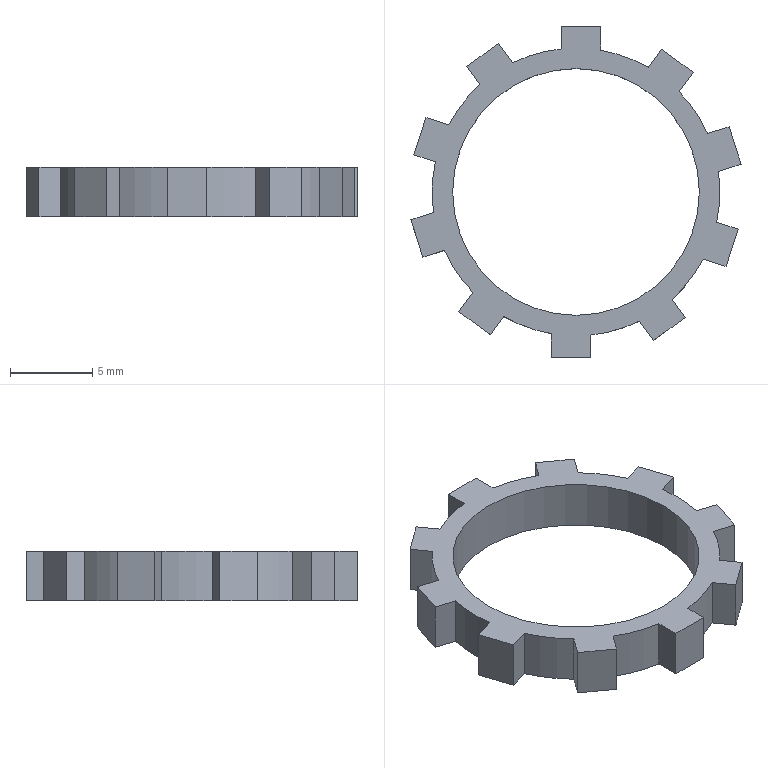Part | NX | features DATUM_CSYS 2, EXTRUDE 1, SKETCH 1 | 1 solid | 43 faces | box 20.095 x 20.159 x 3 mm | volume 289.163 mm3 | plane 32 | cylinder 11 | commonest cylinder face diameters 17.5 x10 15 x1
STEP:
#1=CARTESIAN_POINT('',(-10.047,-1.695,0.));
#2=VERTEX_POINT('',#1);
#3=CARTESIAN_POINT('',(-9.308,-3.971,0.));
#4=VERTEX_POINT('',#3);
#5=CARTESIAN_POINT('',(-10.047,-1.695,0.));
#6=DIRECTION('',(0.309,-0.9511,0.));
#7=VECTOR('',#6,1000.);
#8=LINE('',#5,#7);
#9=EDGE_CURVE('',#2,#4,#8,.T.);
#10=ORIENTED_EDGE('',*,*,#9,.T.);
#11=CARTESIAN_POINT('',(-9.308,-3.971,3.));
#12=VERTEX_POINT('',#11);
#13=CARTESIAN_POINT('',(-9.308,-3.971,3.));
#14=DIRECTION('',(0.,0.,-1.));
#15=VECTOR('',#14,1000.);
#16=LINE('',#13,#15);
#17=EDGE_CURVE('',#12,#4,#16,.T.);
#18=ORIENTED_EDGE('',*,*,#17,.F.);
#19=CARTESIAN_POINT('',(-10.047,-1.695,3.));
#20=VERTEX_POINT('',#19);
#21=CARTESIAN_POINT('',(-10.047,-1.695,3.));
#22=DIRECTION('',(0.309,-0.9511,0.));
#23=VECTOR('',#22,1000.);
#24=LINE('',#21,#23);
#25=EDGE_CURVE('',#20,#12,#24,.T.);
#26=ORIENTED_EDGE('',*,*,#25,.F.);
#27=CARTESIAN_POINT('',(-10.047,-1.695,3.));
#28=DIRECTION('',(0.,0.,-1.));
#29=VECTOR('',#28,1000.);
#30=LINE('',#27,#29);
#31=EDGE_CURVE('',#20,#2,#30,.T.);
#32=ORIENTED_EDGE('',*,*,#31,.T.);
#33=EDGE_LOOP('',(#10,#18,#26,#32));
#34=FACE_BOUND('',#33,.T.);
#35=CARTESIAN_POINT('',(-10.047,-1.695,3.));
#36=DIRECTION('',(0.9511,0.309,0.));
#37=DIRECTION('',(-0.309,0.9511,0.));
#38=AXIS2_PLACEMENT_3D('',#35,#36,#37);
#39=PLANE('',#38);
#40=ADVANCED_FACE('',(#34),#39,.F.);
#41=CARTESIAN_POINT('',(-7.999,-3.545,0.));
#42=VERTEX_POINT('',#41);
#43=CARTESIAN_POINT('',(-9.308,-3.971,0.));
#44=DIRECTION('',(0.9511,0.309,0.));
#45=VECTOR('',#44,1000.);
#46=LINE('',#43,#45);
#47=EDGE_CURVE('',#4,#42,#46,.T.);
#48=ORIENTED_EDGE('',*,*,#47,.T.);
#49=CARTESIAN_POINT('',(-7.999,-3.545,3.));
#50=VERTEX_POINT('',#49);
#51=CARTESIAN_POINT('',(-7.999,-3.545,3.));
#52=DIRECTION('',(0.,0.,-1.));
#53=VECTOR('',#52,1000.);
#54=LINE('',#51,#53);
#55=EDGE_CURVE('',#50,#42,#54,.T.);
#56=ORIENTED_EDGE('',*,*,#55,.F.);
#57=CARTESIAN_POINT('',(-9.308,-3.971,3.));
#58=DIRECTION('',(0.9511,0.309,0.));
#59=VECTOR('',#58,1000.);
#60=LINE('',#57,#59);
#61=EDGE_CURVE('',#12,#50,#60,.T.);
#62=ORIENTED_EDGE('',*,*,#61,.F.);
#63=ORIENTED_EDGE('',*,*,#17,.T.);
#64=EDGE_LOOP('',(#48,#56,#62,#63));
#65=FACE_BOUND('',#64,.T.);
#66=CARTESIAN_POINT('',(-9.308,-3.971,3.));
#67=DIRECTION('',(-0.309,0.9511,0.));
#68=DIRECTION('',(-0.9511,-0.309,0.));
#69=AXIS2_PLACEMENT_3D('',#66,#67,#68);
#70=PLANE('',#69);
#71=ADVANCED_FACE('',(#65),#70,.F.);
#72=CARTESIAN_POINT('',(-6.275,-6.098,0.));
#73=VERTEX_POINT('',#72);
#74=CARTESIAN_POINT('',(0.,0.,0.));
#75=DIRECTION('',(0.,0.,1.));
#76=DIRECTION('',(1.,0.,0.));
#77=AXIS2_PLACEMENT_3D('',#74,#75,#76);
#78=CIRCLE('',#77,8.75);
#79=EDGE_CURVE('',#42,#73,#78,.T.);
#80=ORIENTED_EDGE('',*,*,#79,.T.);
#81=CARTESIAN_POINT('',(-6.275,-6.098,3.));
#82=VERTEX_POINT('',#81);
#83=CARTESIAN_POINT('',(-6.275,-6.098,3.));
#84=DIRECTION('',(0.,0.,-1.));
#85=VECTOR('',#84,1000.);
#86=LINE('',#83,#85);
#87=EDGE_CURVE('',#82,#73,#86,.T.);
#88=ORIENTED_EDGE('',*,*,#87,.F.);
#89=CARTESIAN_POINT('',(0.,0.,3.));
#90=DIRECTION('',(0.,0.,1.));
#91=DIRECTION('',(1.,0.,0.));
#92=AXIS2_PLACEMENT_3D('',#89,#90,#91);
#93=CIRCLE('',#92,8.75);
#94=EDGE_CURVE('',#50,#82,#93,.T.);
#95=ORIENTED_EDGE('',*,*,#94,.F.);
#96=ORIENTED_EDGE('',*,*,#55,.T.);
#97=EDGE_LOOP('',(#80,#88,#95,#96));
#98=FACE_BOUND('',#97,.T.);
#99=CARTESIAN_POINT('',(0.,0.,3.));
#100=DIRECTION('',(0.,0.,-1.));
#101=DIRECTION('',(-1.,0.,0.));
#102=AXIS2_PLACEMENT_3D('',#99,#100,#101);
#103=CYLINDRICAL_SURFACE('',#102,8.75);
#104=ADVANCED_FACE('',(#98),#103,.T.);
#105=CARTESIAN_POINT('',(-7.132,-7.277,0.));
#106=VERTEX_POINT('',#105);
#107=CARTESIAN_POINT('',(-6.275,-6.098,0.));
#108=DIRECTION('',(-0.5878,-0.809,0.));
#109=VECTOR('',#108,1000.);
#110=LINE('',#107,#109);
#111=EDGE_CURVE('',#73,#106,#110,.T.);
#112=ORIENTED_EDGE('',*,*,#111,.T.);
#113=CARTESIAN_POINT('',(-7.132,-7.277,3.));
#114=VERTEX_POINT('',#113);
#115=CARTESIAN_POINT('',(-7.132,-7.277,3.));
#116=DIRECTION('',(0.,0.,-1.));
#117=VECTOR('',#116,1000.);
#118=LINE('',#115,#117);
#119=EDGE_CURVE('',#114,#106,#118,.T.);
#120=ORIENTED_EDGE('',*,*,#119,.F.);
#121=CARTESIAN_POINT('',(-6.275,-6.098,3.));
#122=DIRECTION('',(-0.5878,-0.809,0.));
#123=VECTOR('',#122,1000.);
#124=LINE('',#121,#123);
#125=EDGE_CURVE('',#82,#114,#124,.T.);
#126=ORIENTED_EDGE('',*,*,#125,.F.);
#127=ORIENTED_EDGE('',*,*,#87,.T.);
#128=EDGE_LOOP('',(#112,#120,#126,#127));
#129=FACE_BOUND('',#128,.T.);
#130=CARTESIAN_POINT('',(-6.275,-6.098,3.));
#131=DIRECTION('',(0.809,-0.5878,0.));
#132=DIRECTION('',(0.5878,0.809,0.));
#133=AXIS2_PLACEMENT_3D('',#130,#131,#132);
#134=PLANE('',#133);
#135=ADVANCED_FACE('',(#129),#134,.F.);
#136=CARTESIAN_POINT('',(-5.196,-8.683,0.));
#137=VERTEX_POINT('',#136);
#138=CARTESIAN_POINT('',(-7.132,-7.277,0.));
#139=DIRECTION('',(0.809,-0.5878,0.));
#140=VECTOR('',#139,1000.);
#141=LINE('',#138,#140);
#142=EDGE_CURVE('',#106,#137,#141,.T.);
#143=ORIENTED_EDGE('',*,*,#142,.T.);
#144=CARTESIAN_POINT('',(-5.196,-8.683,3.));
#145=VERTEX_POINT('',#144);
#146=CARTESIAN_POINT('',(-5.196,-8.683,3.));
#147=DIRECTION('',(0.,0.,-1.));
#148=VECTOR('',#147,1000.);
#149=LINE('',#146,#148);
#150=EDGE_CURVE('',#145,#137,#149,.T.);
#151=ORIENTED_EDGE('',*,*,#150,.F.);
#152=CARTESIAN_POINT('',(-7.132,-7.277,3.));
#153=DIRECTION('',(0.809,-0.5878,0.));
#154=VECTOR('',#153,1000.);
#155=LINE('',#152,#154);
#156=EDGE_CURVE('',#114,#145,#155,.T.);
#157=ORIENTED_EDGE('',*,*,#156,.F.);
#158=ORIENTED_EDGE('',*,*,#119,.T.);
#159=EDGE_LOOP('',(#143,#151,#157,#158));
#160=FACE_BOUND('',#159,.T.);
#161=CARTESIAN_POINT('',(-7.132,-7.277,3.));
#162=DIRECTION('',(0.5878,0.809,0.));
#163=DIRECTION('',(-0.809,0.5878,0.));
#164=AXIS2_PLACEMENT_3D('',#161,#162,#163);
#165=PLANE('',#164);
#166=ADVANCED_FACE('',(#160),#165,.F.);
#167=CARTESIAN_POINT('',(-4.388,-7.57,0.));
#168=VERTEX_POINT('',#167);
#169=CARTESIAN_POINT('',(-5.196,-8.683,0.));
#170=DIRECTION('',(0.5878,0.809,0.));
#171=VECTOR('',#170,1000.);
#172=LINE('',#169,#171);
#173=EDGE_CURVE('',#137,#168,#172,.T.);
#174=ORIENTED_EDGE('',*,*,#173,.T.);
#175=CARTESIAN_POINT('',(-4.388,-7.57,3.));
#176=VERTEX_POINT('',#175);
#177=CARTESIAN_POINT('',(-4.388,-7.57,3.));
#178=DIRECTION('',(0.,0.,-1.));
#179=VECTOR('',#178,1000.);
#180=LINE('',#177,#179);
#181=EDGE_CURVE('',#176,#168,#180,.T.);
#182=ORIENTED_EDGE('',*,*,#181,.F.);
#183=CARTESIAN_POINT('',(-5.196,-8.683,3.));
#184=DIRECTION('',(0.5878,0.809,0.));
#185=VECTOR('',#184,1000.);
#186=LINE('',#183,#185);
#187=EDGE_CURVE('',#145,#176,#186,.T.);
#188=ORIENTED_EDGE('',*,*,#187,.F.);
#189=ORIENTED_EDGE('',*,*,#150,.T.);
#190=EDGE_LOOP('',(#174,#182,#188,#189));
#191=FACE_BOUND('',#190,.T.);
#192=CARTESIAN_POINT('',(-5.196,-8.683,3.));
#193=DIRECTION('',(-0.809,0.5878,0.));
#194=DIRECTION('',(-0.5878,-0.809,0.));
#195=AXIS2_PLACEMENT_3D('',#192,#193,#194);
#196=PLANE('',#195);
#197=ADVANCED_FACE('',(#191),#196,.F.);
#198=CARTESIAN_POINT('',(-1.492,-8.622,0.));
#199=VERTEX_POINT('',#198);
#200=CARTESIAN_POINT('',(0.,0.,0.));
#201=DIRECTION('',(0.,0.,1.));
#202=DIRECTION('',(1.,0.,0.));
#203=AXIS2_PLACEMENT_3D('',#200,#201,#202);
#204=CIRCLE('',#203,8.75);
#205=EDGE_CURVE('',#168,#199,#204,.T.);
#206=ORIENTED_EDGE('',*,*,#205,.T.);
#207=CARTESIAN_POINT('',(-1.492,-8.622,3.));
#208=VERTEX_POINT('',#207);
#209=CARTESIAN_POINT('',(-1.492,-8.622,3.));
#210=DIRECTION('',(0.,0.,-1.));
#211=VECTOR('',#210,1000.);
#212=LINE('',#209,#211);
#213=EDGE_CURVE('',#208,#199,#212,.T.);
#214=ORIENTED_EDGE('',*,*,#213,.F.);
#215=CARTESIAN_POINT('',(0.,0.,3.));
#216=DIRECTION('',(0.,0.,1.));
#217=DIRECTION('',(1.,0.,0.));
#218=AXIS2_PLACEMENT_3D('',#215,#216,#217);
#219=CIRCLE('',#218,8.75);
#220=EDGE_CURVE('',#176,#208,#219,.T.);
#221=ORIENTED_EDGE('',*,*,#220,.F.);
#222=ORIENTED_EDGE('',*,*,#181,.T.);
#223=EDGE_LOOP('',(#206,#214,#221,#222));
#224=FACE_BOUND('',#223,.T.);
#225=CARTESIAN_POINT('',(0.,0.,3.));
#226=DIRECTION('',(0.,0.,-1.));
#227=DIRECTION('',(-1.,0.,0.));
#228=AXIS2_PLACEMENT_3D('',#225,#226,#227);
#229=CYLINDRICAL_SURFACE('',#228,8.75);
#230=ADVANCED_FACE('',(#224),#229,.T.);
#231=CARTESIAN_POINT('',(-1.492,-10.079,0.));
#232=VERTEX_POINT('',#231);
#233=CARTESIAN_POINT('',(-1.492,-8.622,0.));
#234=DIRECTION('',(0.,-1.,0.));
#235=VECTOR('',#234,1000.);
#236=LINE('',#233,#235);
#237=EDGE_CURVE('',#199,#232,#236,.T.);
#238=ORIENTED_EDGE('',*,*,#237,.T.);
#239=CARTESIAN_POINT('',(-1.492,-10.079,3.));
#240=VERTEX_POINT('',#239);
#241=CARTESIAN_POINT('',(-1.492,-10.079,3.));
#242=DIRECTION('',(0.,0.,-1.));
#243=VECTOR('',#242,1000.);
#244=LINE('',#241,#243);
#245=EDGE_CURVE('',#240,#232,#244,.T.);
#246=ORIENTED_EDGE('',*,*,#245,.F.);
#247=CARTESIAN_POINT('',(-1.492,-8.622,3.));
#248=DIRECTION('',(0.,-1.,0.));
#249=VECTOR('',#248,1000.);
#250=LINE('',#247,#249);
#251=EDGE_CURVE('',#208,#240,#250,.T.);
#252=ORIENTED_EDGE('',*,*,#251,.F.);
#253=ORIENTED_EDGE('',*,*,#213,.T.);
#254=EDGE_LOOP('',(#238,#246,#252,#253));
#255=FACE_BOUND('',#254,.T.);
#256=CARTESIAN_POINT('',(-1.492,-8.622,3.));
#257=DIRECTION('',(1.,0.,0.));
#258=DIRECTION('',(0.,1.,0.));
#259=AXIS2_PLACEMENT_3D('',#256,#257,#258);
#260=PLANE('',#259);
#261=ADVANCED_FACE('',(#255),#260,.F.);
#262=CARTESIAN_POINT('',(0.9,-10.079,0.));
#263=VERTEX_POINT('',#262);
#264=CARTESIAN_POINT('',(-1.492,-10.079,0.));
#265=DIRECTION('',(1.,0.,0.));
#266=VECTOR('',#265,1000.);
#267=LINE('',#264,#266);
#268=EDGE_CURVE('',#232,#263,#267,.T.);
#269=ORIENTED_EDGE('',*,*,#268,.T.);
#270=CARTESIAN_POINT('',(0.9,-10.079,3.));
#271=VERTEX_POINT('',#270);
#272=CARTESIAN_POINT('',(0.9,-10.079,3.));
#273=DIRECTION('',(0.,0.,-1.));
#274=VECTOR('',#273,1000.);
#275=LINE('',#272,#274);
#276=EDGE_CURVE('',#271,#263,#275,.T.);
#277=ORIENTED_EDGE('',*,*,#276,.F.);
#278=CARTESIAN_POINT('',(-1.492,-10.079,3.));
#279=DIRECTION('',(1.,0.,0.));
#280=VECTOR('',#279,1000.);
#281=LINE('',#278,#280);
#282=EDGE_CURVE('',#240,#271,#281,.T.);
#283=ORIENTED_EDGE('',*,*,#282,.F.);
#284=ORIENTED_EDGE('',*,*,#245,.T.);
#285=EDGE_LOOP('',(#269,#277,#283,#284));
#286=FACE_BOUND('',#285,.T.);
#287=CARTESIAN_POINT('',(-1.492,-10.079,3.));
#288=DIRECTION('',(0.,1.,0.));
#289=DIRECTION('',(0.,0.,1.));
#290=AXIS2_PLACEMENT_3D('',#287,#288,#289);
#291=PLANE('',#290);
#292=ADVANCED_FACE('',(#286),#291,.F.);
#293=CARTESIAN_POINT('',(0.9,-8.703,0.));
#294=VERTEX_POINT('',#293);
#295=CARTESIAN_POINT('',(0.9,-10.079,0.));
#296=DIRECTION('',(0.,1.,0.));
#297=VECTOR('',#296,1000.);
#298=LINE('',#295,#297);
#299=EDGE_CURVE('',#263,#294,#298,.T.);
#300=ORIENTED_EDGE('',*,*,#299,.T.);
#301=CARTESIAN_POINT('',(0.9,-8.703,3.));
#302=VERTEX_POINT('',#301);
#303=CARTESIAN_POINT('',(0.9,-8.703,3.));
#304=DIRECTION('',(0.,0.,-1.));
#305=VECTOR('',#304,1000.);
#306=LINE('',#303,#305);
#307=EDGE_CURVE('',#302,#294,#306,.T.);
#308=ORIENTED_EDGE('',*,*,#307,.F.);
#309=CARTESIAN_POINT('',(0.9,-10.079,3.));
#310=DIRECTION('',(0.,1.,0.));
#311=VECTOR('',#310,1000.);
#312=LINE('',#309,#311);
#313=EDGE_CURVE('',#271,#302,#312,.T.);
#314=ORIENTED_EDGE('',*,*,#313,.F.);
#315=ORIENTED_EDGE('',*,*,#276,.T.);
#316=EDGE_LOOP('',(#300,#308,#314,#315));
#317=FACE_BOUND('',#316,.T.);
#318=CARTESIAN_POINT('',(0.9,-10.079,3.));
#319=DIRECTION('',(-1.,0.,0.));
#320=DIRECTION('',(0.,-1.,0.));
#321=AXIS2_PLACEMENT_3D('',#318,#319,#320);
#322=PLANE('',#321);
#323=ADVANCED_FACE('',(#317),#322,.F.);
#324=CARTESIAN_POINT('',(3.86,-7.852,0.));
#325=VERTEX_POINT('',#324);
#326=CARTESIAN_POINT('',(0.,0.,0.));
#327=DIRECTION('',(0.,0.,1.));
#328=DIRECTION('',(1.,0.,0.));
#329=AXIS2_PLACEMENT_3D('',#326,#327,#328);
#330=CIRCLE('',#329,8.75);
#331=EDGE_CURVE('',#294,#325,#330,.T.);
#332=ORIENTED_EDGE('',*,*,#331,.T.);
#333=CARTESIAN_POINT('',(3.86,-7.852,3.));
#334=VERTEX_POINT('',#333);
#335=CARTESIAN_POINT('',(3.86,-7.852,3.));
#336=DIRECTION('',(0.,0.,-1.));
#337=VECTOR('',#336,1000.);
#338=LINE('',#335,#337);
#339=EDGE_CURVE('',#334,#325,#338,.T.);
#340=ORIENTED_EDGE('',*,*,#339,.F.);
#341=CARTESIAN_POINT('',(0.,0.,3.));
#342=DIRECTION('',(0.,0.,1.));
#343=DIRECTION('',(1.,0.,0.));
#344=AXIS2_PLACEMENT_3D('',#341,#342,#343);
#345=CIRCLE('',#344,8.75);
#346=EDGE_CURVE('',#302,#334,#345,.T.);
#347=ORIENTED_EDGE('',*,*,#346,.F.);
#348=ORIENTED_EDGE('',*,*,#307,.T.);
#349=EDGE_LOOP('',(#332,#340,#347,#348));
#350=FACE_BOUND('',#349,.T.);
#351=CARTESIAN_POINT('',(0.,0.,3.));
#352=DIRECTION('',(0.,0.,-1.));
#353=DIRECTION('',(-1.,0.,0.));
#354=AXIS2_PLACEMENT_3D('',#351,#352,#353);
#355=CYLINDRICAL_SURFACE('',#354,8.75);
#356=ADVANCED_FACE('',(#350),#355,.T.);
#357=CARTESIAN_POINT('',(4.717,-9.032,0.));
#358=VERTEX_POINT('',#357);
#359=CARTESIAN_POINT('',(3.86,-7.852,0.));
#360=DIRECTION('',(0.5878,-0.809,0.));
#361=VECTOR('',#360,1000.);
#362=LINE('',#359,#361);
#363=EDGE_CURVE('',#325,#358,#362,.T.);
#364=ORIENTED_EDGE('',*,*,#363,.T.);
#365=CARTESIAN_POINT('',(4.717,-9.032,3.));
#366=VERTEX_POINT('',#365);
#367=CARTESIAN_POINT('',(4.717,-9.032,3.));
#368=DIRECTION('',(0.,0.,-1.));
#369=VECTOR('',#368,1000.);
#370=LINE('',#367,#369);
#371=EDGE_CURVE('',#366,#358,#370,.T.);
#372=ORIENTED_EDGE('',*,*,#371,.F.);
#373=CARTESIAN_POINT('',(3.86,-7.852,3.));
#374=DIRECTION('',(0.5878,-0.809,0.));
#375=VECTOR('',#374,1000.);
#376=LINE('',#373,#375);
#377=EDGE_CURVE('',#334,#366,#376,.T.);
#378=ORIENTED_EDGE('',*,*,#377,.F.);
#379=ORIENTED_EDGE('',*,*,#339,.T.);
#380=EDGE_LOOP('',(#364,#372,#378,#379));
#381=FACE_BOUND('',#380,.T.);
#382=CARTESIAN_POINT('',(3.86,-7.852,3.));
#383=DIRECTION('',(0.809,0.5878,0.));
#384=DIRECTION('',(-0.5878,0.809,0.));
#385=AXIS2_PLACEMENT_3D('',#382,#383,#384);
#386=PLANE('',#385);
#387=ADVANCED_FACE('',(#381),#386,.F.);
#388=CARTESIAN_POINT('',(6.653,-7.625,0.));
#389=VERTEX_POINT('',#388);
#390=CARTESIAN_POINT('',(4.717,-9.032,0.));
#391=DIRECTION('',(0.809,0.5878,0.));
#392=VECTOR('',#391,1000.);
#393=LINE('',#390,#392);
#394=EDGE_CURVE('',#358,#389,#393,.T.);
#395=ORIENTED_EDGE('',*,*,#394,.T.);
#396=CARTESIAN_POINT('',(6.653,-7.625,3.));
#397=VERTEX_POINT('',#396);
#398=CARTESIAN_POINT('',(6.653,-7.625,3.));
#399=DIRECTION('',(0.,0.,-1.));
#400=VECTOR('',#399,1000.);
#401=LINE('',#398,#400);
#402=EDGE_CURVE('',#397,#389,#401,.T.);
#403=ORIENTED_EDGE('',*,*,#402,.F.);
#404=CARTESIAN_POINT('',(4.717,-9.032,3.));
#405=DIRECTION('',(0.809,0.5878,0.));
#406=VECTOR('',#405,1000.);
#407=LINE('',#404,#406);
#408=EDGE_CURVE('',#366,#397,#407,.T.);
#409=ORIENTED_EDGE('',*,*,#408,.F.);
#410=ORIENTED_EDGE('',*,*,#371,.T.);
#411=EDGE_LOOP('',(#395,#403,#409,#410));
#412=FACE_BOUND('',#411,.T.);
#413=CARTESIAN_POINT('',(4.717,-9.032,3.));
#414=DIRECTION('',(-0.5878,0.809,0.));
#415=DIRECTION('',(-0.809,-0.5878,0.));
#416=AXIS2_PLACEMENT_3D('',#413,#414,#415);
#417=PLANE('',#416);
#418=ADVANCED_FACE('',(#412),#417,.F.);
#419=CARTESIAN_POINT('',(5.844,-6.512,0.));
#420=VERTEX_POINT('',#419);
#421=CARTESIAN_POINT('',(6.653,-7.625,0.));
#422=DIRECTION('',(-0.5878,0.809,0.));
#423=VECTOR('',#422,1000.);
#424=LINE('',#421,#423);
#425=EDGE_CURVE('',#389,#420,#424,.T.);
#426=ORIENTED_EDGE('',*,*,#425,.T.);
#427=CARTESIAN_POINT('',(5.844,-6.512,3.));
#428=VERTEX_POINT('',#427);
#429=CARTESIAN_POINT('',(5.844,-6.512,3.));
#430=DIRECTION('',(0.,0.,-1.));
#431=VECTOR('',#430,1000.);
#432=LINE('',#429,#431);
#433=EDGE_CURVE('',#428,#420,#432,.T.);
#434=ORIENTED_EDGE('',*,*,#433,.F.);
#435=CARTESIAN_POINT('',(6.653,-7.625,3.));
#436=DIRECTION('',(-0.5878,0.809,0.));
#437=VECTOR('',#436,1000.);
#438=LINE('',#435,#437);
#439=EDGE_CURVE('',#397,#428,#438,.T.);
#440=ORIENTED_EDGE('',*,*,#439,.F.);
#441=ORIENTED_EDGE('',*,*,#402,.T.);
#442=EDGE_LOOP('',(#426,#434,#440,#441));
#443=FACE_BOUND('',#442,.T.);
#444=CARTESIAN_POINT('',(6.653,-7.625,3.));
#445=DIRECTION('',(-0.809,-0.5878,0.));
#446=DIRECTION('',(0.5878,-0.809,0.));
#447=AXIS2_PLACEMENT_3D('',#444,#445,#446);
#448=PLANE('',#447);
#449=ADVANCED_FACE('',(#443),#448,.F.);
#450=CARTESIAN_POINT('',(7.738,-4.084,0.));
#451=VERTEX_POINT('',#450);
#452=CARTESIAN_POINT('',(0.,0.,0.));
#453=DIRECTION('',(0.,0.,1.));
#454=DIRECTION('',(1.,0.,0.));
#455=AXIS2_PLACEMENT_3D('',#452,#453,#454);
#456=CIRCLE('',#455,8.75);
#457=EDGE_CURVE('',#420,#451,#456,.T.);
#458=ORIENTED_EDGE('',*,*,#457,.T.);
#459=CARTESIAN_POINT('',(7.738,-4.084,3.));
#460=VERTEX_POINT('',#459);
#461=CARTESIAN_POINT('',(7.738,-4.084,3.));
#462=DIRECTION('',(0.,0.,-1.));
#463=VECTOR('',#462,1000.);
#464=LINE('',#461,#463);
#465=EDGE_CURVE('',#460,#451,#464,.T.);
#466=ORIENTED_EDGE('',*,*,#465,.F.);
#467=CARTESIAN_POINT('',(0.,0.,3.));
#468=DIRECTION('',(0.,0.,1.));
#469=DIRECTION('',(1.,0.,0.));
#470=AXIS2_PLACEMENT_3D('',#467,#468,#469);
#471=CIRCLE('',#470,8.75);
#472=EDGE_CURVE('',#428,#460,#471,.T.);
#473=ORIENTED_EDGE('',*,*,#472,.F.);
#474=ORIENTED_EDGE('',*,*,#433,.T.);
#475=EDGE_LOOP('',(#458,#466,#473,#474));
#476=FACE_BOUND('',#475,.T.);
#477=CARTESIAN_POINT('',(0.,0.,3.));
#478=DIRECTION('',(0.,0.,-1.));
#479=DIRECTION('',(-1.,0.,0.));
#480=AXIS2_PLACEMENT_3D('',#477,#478,#479);
#481=CYLINDRICAL_SURFACE('',#480,8.75);
#482=ADVANCED_FACE('',(#476),#481,.T.);
#483=CARTESIAN_POINT('',(9.125,-4.534,0.));
#484=VERTEX_POINT('',#483);
#485=CARTESIAN_POINT('',(7.738,-4.084,0.));
#486=DIRECTION('',(0.9511,-0.309,0.));
#487=VECTOR('',#486,1000.);
#488=LINE('',#485,#487);
#489=EDGE_CURVE('',#451,#484,#488,.T.);
#490=ORIENTED_EDGE('',*,*,#489,.T.);
#491=CARTESIAN_POINT('',(9.125,-4.534,3.));
#492=VERTEX_POINT('',#491);
#493=CARTESIAN_POINT('',(9.125,-4.534,3.));
#494=DIRECTION('',(0.,0.,-1.));
#495=VECTOR('',#494,1000.);
#496=LINE('',#493,#495);
#497=EDGE_CURVE('',#492,#484,#496,.T.);
#498=ORIENTED_EDGE('',*,*,#497,.F.);
#499=CARTESIAN_POINT('',(7.738,-4.084,3.));
#500=DIRECTION('',(0.9511,-0.309,0.));
#501=VECTOR('',#500,1000.);
#502=LINE('',#499,#501);
#503=EDGE_CURVE('',#460,#492,#502,.T.);
#504=ORIENTED_EDGE('',*,*,#503,.F.);
#505=ORIENTED_EDGE('',*,*,#465,.T.);
#506=EDGE_LOOP('',(#490,#498,#504,#505));
#507=FACE_BOUND('',#506,.T.);
#508=CARTESIAN_POINT('',(7.738,-4.084,3.));
#509=DIRECTION('',(0.309,0.9511,0.));
#510=DIRECTION('',(-0.9511,0.309,0.));
#511=AXIS2_PLACEMENT_3D('',#508,#509,#510);
#512=PLANE('',#511);
#513=ADVANCED_FACE('',(#507),#512,.F.);
#514=CARTESIAN_POINT('',(9.864,-2.259,0.));
#515=VERTEX_POINT('',#514);
#516=CARTESIAN_POINT('',(9.125,-4.534,0.));
#517=DIRECTION('',(0.309,0.9511,0.));
#518=VECTOR('',#517,1000.);
#519=LINE('',#516,#518);
#520=EDGE_CURVE('',#484,#515,#519,.T.);
#521=ORIENTED_EDGE('',*,*,#520,.T.);
#522=CARTESIAN_POINT('',(9.864,-2.259,3.));
#523=VERTEX_POINT('',#522);
#524=CARTESIAN_POINT('',(9.864,-2.259,3.));
#525=DIRECTION('',(0.,0.,-1.));
#526=VECTOR('',#525,1000.);
#527=LINE('',#524,#526);
#528=EDGE_CURVE('',#523,#515,#527,.T.);
#529=ORIENTED_EDGE('',*,*,#528,.F.);
#530=CARTESIAN_POINT('',(9.125,-4.534,3.));
#531=DIRECTION('',(0.309,0.9511,0.));
#532=VECTOR('',#531,1000.);
#533=LINE('',#530,#532);
#534=EDGE_CURVE('',#492,#523,#533,.T.);
#535=ORIENTED_EDGE('',*,*,#534,.F.);
#536=ORIENTED_EDGE('',*,*,#497,.T.);
#537=EDGE_LOOP('',(#521,#529,#535,#536));
#538=FACE_BOUND('',#537,.T.);
#539=CARTESIAN_POINT('',(9.125,-4.534,3.));
#540=DIRECTION('',(-0.9511,0.309,0.));
#541=DIRECTION('',(-0.309,-0.9511,0.));
#542=AXIS2_PLACEMENT_3D('',#539,#540,#541);
#543=PLANE('',#542);
#544=ADVANCED_FACE('',(#538),#543,.F.);
#545=CARTESIAN_POINT('',(8.555,-1.834,0.));
#546=VERTEX_POINT('',#545);
#547=CARTESIAN_POINT('',(9.864,-2.259,0.));
#548=DIRECTION('',(-0.9511,0.309,0.));
#549=VECTOR('',#548,1000.);
#550=LINE('',#547,#549);
#551=EDGE_CURVE('',#515,#546,#550,.T.);
#552=ORIENTED_EDGE('',*,*,#551,.T.);
#553=CARTESIAN_POINT('',(8.555,-1.834,3.));
#554=VERTEX_POINT('',#553);
#555=CARTESIAN_POINT('',(8.555,-1.834,3.));
#556=DIRECTION('',(0.,0.,-1.));
#557=VECTOR('',#556,1000.);
#558=LINE('',#555,#557);
#559=EDGE_CURVE('',#554,#546,#558,.T.);
#560=ORIENTED_EDGE('',*,*,#559,.F.);
#561=CARTESIAN_POINT('',(9.864,-2.259,3.));
#562=DIRECTION('',(-0.9511,0.309,0.));
#563=VECTOR('',#562,1000.);
#564=LINE('',#561,#563);
#565=EDGE_CURVE('',#523,#554,#564,.T.);
#566=ORIENTED_EDGE('',*,*,#565,.F.);
#567=ORIENTED_EDGE('',*,*,#528,.T.);
#568=EDGE_LOOP('',(#552,#560,#566,#567));
#569=FACE_BOUND('',#568,.T.);
#570=CARTESIAN_POINT('',(9.864,-2.259,3.));
#571=DIRECTION('',(-0.309,-0.9511,0.));
#572=DIRECTION('',(0.9511,-0.309,0.));
#573=AXIS2_PLACEMENT_3D('',#570,#571,#572);
#574=PLANE('',#573);
#575=ADVANCED_FACE('',(#569),#574,.F.);
#576=CARTESIAN_POINT('',(8.661,1.245,0.));
#577=VERTEX_POINT('',#576);
#578=CARTESIAN_POINT('',(0.,0.,0.));
#579=DIRECTION('',(0.,0.,1.));
#580=DIRECTION('',(1.,0.,0.));
#581=AXIS2_PLACEMENT_3D('',#578,#579,#580);
#582=CIRCLE('',#581,8.75);
#583=EDGE_CURVE('',#546,#577,#582,.T.);
#584=ORIENTED_EDGE('',*,*,#583,.T.);
#585=CARTESIAN_POINT('',(8.661,1.245,3.));
#586=VERTEX_POINT('',#585);
#587=CARTESIAN_POINT('',(8.661,1.245,3.));
#588=DIRECTION('',(0.,0.,-1.));
#589=VECTOR('',#588,1000.);
#590=LINE('',#587,#589);
#591=EDGE_CURVE('',#586,#577,#590,.T.);
#592=ORIENTED_EDGE('',*,*,#591,.F.);
#593=CARTESIAN_POINT('',(0.,0.,3.));
#594=DIRECTION('',(0.,0.,1.));
#595=DIRECTION('',(1.,0.,0.));
#596=AXIS2_PLACEMENT_3D('',#593,#594,#595);
#597=CIRCLE('',#596,8.75);
#598=EDGE_CURVE('',#554,#586,#597,.T.);
#599=ORIENTED_EDGE('',*,*,#598,.F.);
#600=ORIENTED_EDGE('',*,*,#559,.T.);
#601=EDGE_LOOP('',(#584,#592,#599,#600));
#602=FACE_BOUND('',#601,.T.);
#603=CARTESIAN_POINT('',(0.,0.,3.));
#604=DIRECTION('',(0.,0.,-1.));
#605=DIRECTION('',(-1.,0.,0.));
#606=AXIS2_PLACEMENT_3D('',#603,#604,#605);
#607=CYLINDRICAL_SURFACE('',#606,8.75);
#608=ADVANCED_FACE('',(#602),#607,.T.);
#609=CARTESIAN_POINT('',(10.047,1.695,0.));
#610=VERTEX_POINT('',#609);
#611=CARTESIAN_POINT('',(8.661,1.245,0.));
#612=DIRECTION('',(0.9511,0.309,0.));
#613=VECTOR('',#612,1000.);
#614=LINE('',#611,#613);
#615=EDGE_CURVE('',#577,#610,#614,.T.);
#616=ORIENTED_EDGE('',*,*,#615,.T.);
#617=CARTESIAN_POINT('',(10.047,1.695,3.));
#618=VERTEX_POINT('',#617);
#619=CARTESIAN_POINT('',(10.047,1.695,3.));
#620=DIRECTION('',(0.,0.,-1.));
#621=VECTOR('',#620,1000.);
#622=LINE('',#619,#621);
#623=EDGE_CURVE('',#618,#610,#622,.T.);
#624=ORIENTED_EDGE('',*,*,#623,.F.);
#625=CARTESIAN_POINT('',(8.661,1.245,3.));
#626=DIRECTION('',(0.9511,0.309,0.));
#627=VECTOR('',#626,1000.);
#628=LINE('',#625,#627);
#629=EDGE_CURVE('',#586,#618,#628,.T.);
#630=ORIENTED_EDGE('',*,*,#629,.F.);
#631=ORIENTED_EDGE('',*,*,#591,.T.);
#632=EDGE_LOOP('',(#616,#624,#630,#631));
#633=FACE_BOUND('',#632,.T.);
#634=CARTESIAN_POINT('',(8.661,1.245,3.));
#635=DIRECTION('',(-0.309,0.9511,0.));
#636=DIRECTION('',(-0.9511,-0.309,0.));
#637=AXIS2_PLACEMENT_3D('',#634,#635,#636);
#638=PLANE('',#637);
#639=ADVANCED_FACE('',(#633),#638,.F.);
#640=CARTESIAN_POINT('',(9.308,3.971,0.));
#641=VERTEX_POINT('',#640);
#642=CARTESIAN_POINT('',(10.047,1.695,0.));
#643=DIRECTION('',(-0.309,0.9511,0.));
#644=VECTOR('',#643,1000.);
#645=LINE('',#642,#644);
#646=EDGE_CURVE('',#610,#641,#645,.T.);
#647=ORIENTED_EDGE('',*,*,#646,.T.);
#648=CARTESIAN_POINT('',(9.308,3.971,3.));
#649=VERTEX_POINT('',#648);
#650=CARTESIAN_POINT('',(9.308,3.971,3.));
#651=DIRECTION('',(0.,0.,-1.));
#652=VECTOR('',#651,1000.);
#653=LINE('',#650,#652);
#654=EDGE_CURVE('',#649,#641,#653,.T.);
#655=ORIENTED_EDGE('',*,*,#654,.F.);
#656=CARTESIAN_POINT('',(10.047,1.695,3.));
#657=DIRECTION('',(-0.309,0.9511,0.));
#658=VECTOR('',#657,1000.);
#659=LINE('',#656,#658);
#660=EDGE_CURVE('',#618,#649,#659,.T.);
#661=ORIENTED_EDGE('',*,*,#660,.F.);
#662=ORIENTED_EDGE('',*,*,#623,.T.);
#663=EDGE_LOOP('',(#647,#655,#661,#662));
#664=FACE_BOUND('',#663,.T.);
#665=CARTESIAN_POINT('',(10.047,1.695,3.));
#666=DIRECTION('',(-0.9511,-0.309,0.));
#667=DIRECTION('',(0.309,-0.9511,0.));
#668=AXIS2_PLACEMENT_3D('',#665,#666,#667);
#669=PLANE('',#668);
#670=ADVANCED_FACE('',(#664),#669,.F.);
#671=CARTESIAN_POINT('',(7.999,3.545,0.));
#672=VERTEX_POINT('',#671);
#673=CARTESIAN_POINT('',(9.308,3.971,0.));
#674=DIRECTION('',(-0.9511,-0.309,0.));
#675=VECTOR('',#674,1000.);
#676=LINE('',#673,#675);
#677=EDGE_CURVE('',#641,#672,#676,.T.);
#678=ORIENTED_EDGE('',*,*,#677,.T.);
#679=CARTESIAN_POINT('',(7.999,3.545,3.));
#680=VERTEX_POINT('',#679);
#681=CARTESIAN_POINT('',(7.999,3.545,3.));
#682=DIRECTION('',(0.,0.,-1.));
#683=VECTOR('',#682,1000.);
#684=LINE('',#681,#683);
#685=EDGE_CURVE('',#680,#672,#684,.T.);
#686=ORIENTED_EDGE('',*,*,#685,.F.);
#687=CARTESIAN_POINT('',(9.308,3.971,3.));
#688=DIRECTION('',(-0.9511,-0.309,0.));
#689=VECTOR('',#688,1000.);
#690=LINE('',#687,#689);
#691=EDGE_CURVE('',#649,#680,#690,.T.);
#692=ORIENTED_EDGE('',*,*,#691,.F.);
#693=ORIENTED_EDGE('',*,*,#654,.T.);
#694=EDGE_LOOP('',(#678,#686,#692,#693));
#695=FACE_BOUND('',#694,.T.);
#696=CARTESIAN_POINT('',(9.308,3.971,3.));
#697=DIRECTION('',(0.309,-0.9511,0.));
#698=DIRECTION('',(0.9511,0.309,0.));
#699=AXIS2_PLACEMENT_3D('',#696,#697,#698);
#700=PLANE('',#699);
#701=ADVANCED_FACE('',(#695),#700,.F.);
#702=CARTESIAN_POINT('',(6.275,6.098,0.));
#703=VERTEX_POINT('',#702);
#704=CARTESIAN_POINT('',(0.,0.,0.));
#705=DIRECTION('',(0.,0.,1.));
#706=DIRECTION('',(1.,0.,0.));
#707=AXIS2_PLACEMENT_3D('',#704,#705,#706);
#708=CIRCLE('',#707,8.75);
#709=EDGE_CURVE('',#672,#703,#708,.T.);
#710=ORIENTED_EDGE('',*,*,#709,.T.);
#711=CARTESIAN_POINT('',(6.275,6.098,3.));
#712=VERTEX_POINT('',#711);
#713=CARTESIAN_POINT('',(6.275,6.098,3.));
#714=DIRECTION('',(0.,0.,-1.));
#715=VECTOR('',#714,1000.);
#716=LINE('',#713,#715);
#717=EDGE_CURVE('',#712,#703,#716,.T.);
#718=ORIENTED_EDGE('',*,*,#717,.F.);
#719=CARTESIAN_POINT('',(0.,0.,3.));
#720=DIRECTION('',(0.,0.,1.));
#721=DIRECTION('',(1.,0.,0.));
#722=AXIS2_PLACEMENT_3D('',#719,#720,#721);
#723=CIRCLE('',#722,8.75);
#724=EDGE_CURVE('',#680,#712,#723,.T.);
#725=ORIENTED_EDGE('',*,*,#724,.F.);
#726=ORIENTED_EDGE('',*,*,#685,.T.);
#727=EDGE_LOOP('',(#710,#718,#725,#726));
#728=FACE_BOUND('',#727,.T.);
#729=CARTESIAN_POINT('',(0.,0.,3.));
#730=DIRECTION('',(0.,0.,-1.));
#731=DIRECTION('',(-1.,0.,0.));
#732=AXIS2_PLACEMENT_3D('',#729,#730,#731);
#733=CYLINDRICAL_SURFACE('',#732,8.75);
#734=ADVANCED_FACE('',(#728),#733,.T.);
#735=CARTESIAN_POINT('',(7.132,7.277,0.));
#736=VERTEX_POINT('',#735);
#737=CARTESIAN_POINT('',(6.275,6.098,0.));
#738=DIRECTION('',(0.5878,0.809,0.));
#739=VECTOR('',#738,1000.);
#740=LINE('',#737,#739);
#741=EDGE_CURVE('',#703,#736,#740,.T.);
#742=ORIENTED_EDGE('',*,*,#741,.T.);
#743=CARTESIAN_POINT('',(7.132,7.277,3.));
#744=VERTEX_POINT('',#743);
#745=CARTESIAN_POINT('',(7.132,7.277,3.));
#746=DIRECTION('',(0.,0.,-1.));
#747=VECTOR('',#746,1000.);
#748=LINE('',#745,#747);
#749=EDGE_CURVE('',#744,#736,#748,.T.);
#750=ORIENTED_EDGE('',*,*,#749,.F.);
#751=CARTESIAN_POINT('',(6.275,6.098,3.));
#752=DIRECTION('',(0.5878,0.809,0.));
#753=VECTOR('',#752,1000.);
#754=LINE('',#751,#753);
#755=EDGE_CURVE('',#712,#744,#754,.T.);
#756=ORIENTED_EDGE('',*,*,#755,.F.);
#757=ORIENTED_EDGE('',*,*,#717,.T.);
#758=EDGE_LOOP('',(#742,#750,#756,#757));
#759=FACE_BOUND('',#758,.T.);
#760=CARTESIAN_POINT('',(6.275,6.098,3.));
#761=DIRECTION('',(-0.809,0.5878,0.));
#762=DIRECTION('',(-0.5878,-0.809,0.));
#763=AXIS2_PLACEMENT_3D('',#760,#761,#762);
#764=PLANE('',#763);
#765=ADVANCED_FACE('',(#759),#764,.F.);
#766=CARTESIAN_POINT('',(5.196,8.683,0.));
#767=VERTEX_POINT('',#766);
#768=CARTESIAN_POINT('',(7.132,7.277,0.));
#769=DIRECTION('',(-0.809,0.5878,0.));
#770=VECTOR('',#769,1000.);
#771=LINE('',#768,#770);
#772=EDGE_CURVE('',#736,#767,#771,.T.);
#773=ORIENTED_EDGE('',*,*,#772,.T.);
#774=CARTESIAN_POINT('',(5.196,8.683,3.));
#775=VERTEX_POINT('',#774);
#776=CARTESIAN_POINT('',(5.196,8.683,3.));
#777=DIRECTION('',(0.,0.,-1.));
#778=VECTOR('',#777,1000.);
#779=LINE('',#776,#778);
#780=EDGE_CURVE('',#775,#767,#779,.T.);
#781=ORIENTED_EDGE('',*,*,#780,.F.);
#782=CARTESIAN_POINT('',(7.132,7.277,3.));
#783=DIRECTION('',(-0.809,0.5878,0.));
#784=VECTOR('',#783,1000.);
#785=LINE('',#782,#784);
#786=EDGE_CURVE('',#744,#775,#785,.T.);
#787=ORIENTED_EDGE('',*,*,#786,.F.);
#788=ORIENTED_EDGE('',*,*,#749,.T.);
#789=EDGE_LOOP('',(#773,#781,#787,#788));
#790=FACE_BOUND('',#789,.T.);
#791=CARTESIAN_POINT('',(7.132,7.277,3.));
#792=DIRECTION('',(-0.5878,-0.809,0.));
#793=DIRECTION('',(0.809,-0.5878,0.));
#794=AXIS2_PLACEMENT_3D('',#791,#792,#793);
#795=PLANE('',#794);
#796=ADVANCED_FACE('',(#790),#795,.F.);
#797=CARTESIAN_POINT('',(4.388,7.57,0.));
#798=VERTEX_POINT('',#797);
#799=CARTESIAN_POINT('',(5.196,8.683,0.));
#800=DIRECTION('',(-0.5878,-0.809,0.));
#801=VECTOR('',#800,1000.);
#802=LINE('',#799,#801);
#803=EDGE_CURVE('',#767,#798,#802,.T.);
#804=ORIENTED_EDGE('',*,*,#803,.T.);
#805=CARTESIAN_POINT('',(4.388,7.57,3.));
#806=VERTEX_POINT('',#805);
#807=CARTESIAN_POINT('',(4.388,7.57,3.));
#808=DIRECTION('',(0.,0.,-1.));
#809=VECTOR('',#808,1000.);
#810=LINE('',#807,#809);
#811=EDGE_CURVE('',#806,#798,#810,.T.);
#812=ORIENTED_EDGE('',*,*,#811,.F.);
#813=CARTESIAN_POINT('',(5.196,8.683,3.));
#814=DIRECTION('',(-0.5878,-0.809,0.));
#815=VECTOR('',#814,1000.);
#816=LINE('',#813,#815);
#817=EDGE_CURVE('',#775,#806,#816,.T.);
#818=ORIENTED_EDGE('',*,*,#817,.F.);
#819=ORIENTED_EDGE('',*,*,#780,.T.);
#820=EDGE_LOOP('',(#804,#812,#818,#819));
#821=FACE_BOUND('',#820,.T.);
#822=CARTESIAN_POINT('',(5.196,8.683,3.));
#823=DIRECTION('',(0.809,-0.5878,0.));
#824=DIRECTION('',(0.5878,0.809,0.));
#825=AXIS2_PLACEMENT_3D('',#822,#823,#824);
#826=PLANE('',#825);
#827=ADVANCED_FACE('',(#821),#826,.F.);
#828=CARTESIAN_POINT('',(1.492,8.622,0.));
#829=VERTEX_POINT('',#828);
#830=CARTESIAN_POINT('',(0.,0.,0.));
#831=DIRECTION('',(0.,0.,1.));
#832=DIRECTION('',(1.,0.,0.));
#833=AXIS2_PLACEMENT_3D('',#830,#831,#832);
#834=CIRCLE('',#833,8.75);
#835=EDGE_CURVE('',#798,#829,#834,.T.);
#836=ORIENTED_EDGE('',*,*,#835,.T.);
#837=CARTESIAN_POINT('',(1.492,8.622,3.));
#838=VERTEX_POINT('',#837);
#839=CARTESIAN_POINT('',(1.492,8.622,3.));
#840=DIRECTION('',(0.,0.,-1.));
#841=VECTOR('',#840,1000.);
#842=LINE('',#839,#841);
#843=EDGE_CURVE('',#838,#829,#842,.T.);
#844=ORIENTED_EDGE('',*,*,#843,.F.);
#845=CARTESIAN_POINT('',(0.,0.,3.));
#846=DIRECTION('',(0.,0.,1.));
#847=DIRECTION('',(1.,0.,0.));
#848=AXIS2_PLACEMENT_3D('',#845,#846,#847);
#849=CIRCLE('',#848,8.75);
#850=EDGE_CURVE('',#806,#838,#849,.T.);
#851=ORIENTED_EDGE('',*,*,#850,.F.);
#852=ORIENTED_EDGE('',*,*,#811,.T.);
#853=EDGE_LOOP('',(#836,#844,#851,#852));
#854=FACE_BOUND('',#853,.T.);
#855=CARTESIAN_POINT('',(0.,0.,3.));
#856=DIRECTION('',(0.,0.,-1.));
#857=DIRECTION('',(-1.,0.,0.));
#858=AXIS2_PLACEMENT_3D('',#855,#856,#857);
#859=CYLINDRICAL_SURFACE('',#858,8.75);
#860=ADVANCED_FACE('',(#854),#859,.T.);
#861=CARTESIAN_POINT('',(1.492,10.079,0.));
#862=VERTEX_POINT('',#861);
#863=CARTESIAN_POINT('',(1.492,8.622,0.));
#864=DIRECTION('',(0.,1.,0.));
#865=VECTOR('',#864,1000.);
#866=LINE('',#863,#865);
#867=EDGE_CURVE('',#829,#862,#866,.T.);
#868=ORIENTED_EDGE('',*,*,#867,.T.);
#869=CARTESIAN_POINT('',(1.492,10.079,3.));
#870=VERTEX_POINT('',#869);
#871=CARTESIAN_POINT('',(1.492,10.079,3.));
#872=DIRECTION('',(0.,0.,-1.));
#873=VECTOR('',#872,1000.);
#874=LINE('',#871,#873);
#875=EDGE_CURVE('',#870,#862,#874,.T.);
#876=ORIENTED_EDGE('',*,*,#875,.F.);
#877=CARTESIAN_POINT('',(1.492,8.622,3.));
#878=DIRECTION('',(0.,1.,0.));
#879=VECTOR('',#878,1000.);
#880=LINE('',#877,#879);
#881=EDGE_CURVE('',#838,#870,#880,.T.);
#882=ORIENTED_EDGE('',*,*,#881,.F.);
#883=ORIENTED_EDGE('',*,*,#843,.T.);
#884=EDGE_LOOP('',(#868,#876,#882,#883));
#885=FACE_BOUND('',#884,.T.);
#886=CARTESIAN_POINT('',(1.492,8.622,3.));
#887=DIRECTION('',(-1.,0.,0.));
#888=DIRECTION('',(0.,-1.,0.));
#889=AXIS2_PLACEMENT_3D('',#886,#887,#888);
#890=PLANE('',#889);
#891=ADVANCED_FACE('',(#885),#890,.F.);
#892=CARTESIAN_POINT('',(-0.9,10.079,0.));
#893=VERTEX_POINT('',#892);
#894=CARTESIAN_POINT('',(1.492,10.079,0.));
#895=DIRECTION('',(-1.,0.,0.));
#896=VECTOR('',#895,1000.);
#897=LINE('',#894,#896);
#898=EDGE_CURVE('',#862,#893,#897,.T.);
#899=ORIENTED_EDGE('',*,*,#898,.T.);
#900=CARTESIAN_POINT('',(-0.9,10.079,3.));
#901=VERTEX_POINT('',#900);
#902=CARTESIAN_POINT('',(-0.9,10.079,3.));
#903=DIRECTION('',(0.,0.,-1.));
#904=VECTOR('',#903,1000.);
#905=LINE('',#902,#904);
#906=EDGE_CURVE('',#901,#893,#905,.T.);
#907=ORIENTED_EDGE('',*,*,#906,.F.);
#908=CARTESIAN_POINT('',(1.492,10.079,3.));
#909=DIRECTION('',(-1.,0.,0.));
#910=VECTOR('',#909,1000.);
#911=LINE('',#908,#910);
#912=EDGE_CURVE('',#870,#901,#911,.T.);
#913=ORIENTED_EDGE('',*,*,#912,.F.);
#914=ORIENTED_EDGE('',*,*,#875,.T.);
#915=EDGE_LOOP('',(#899,#907,#913,#914));
#916=FACE_BOUND('',#915,.T.);
#917=CARTESIAN_POINT('',(1.492,10.079,3.));
#918=DIRECTION('',(0.,-1.,0.));
#919=DIRECTION('',(0.,0.,-1.));
#920=AXIS2_PLACEMENT_3D('',#917,#918,#919);
#921=PLANE('',#920);
#922=ADVANCED_FACE('',(#916),#921,.F.);
#923=CARTESIAN_POINT('',(-0.9,8.703,0.));
#924=VERTEX_POINT('',#923);
#925=CARTESIAN_POINT('',(-0.9,10.079,0.));
#926=DIRECTION('',(0.,-1.,0.));
#927=VECTOR('',#926,1000.);
#928=LINE('',#925,#927);
#929=EDGE_CURVE('',#893,#924,#928,.T.);
#930=ORIENTED_EDGE('',*,*,#929,.T.);
#931=CARTESIAN_POINT('',(-0.9,8.703,3.));
#932=VERTEX_POINT('',#931);
#933=CARTESIAN_POINT('',(-0.9,8.703,3.));
#934=DIRECTION('',(0.,0.,-1.));
#935=VECTOR('',#934,1000.);
#936=LINE('',#933,#935);
#937=EDGE_CURVE('',#932,#924,#936,.T.);
#938=ORIENTED_EDGE('',*,*,#937,.F.);
#939=CARTESIAN_POINT('',(-0.9,10.079,3.));
#940=DIRECTION('',(0.,-1.,0.));
#941=VECTOR('',#940,1000.);
#942=LINE('',#939,#941);
#943=EDGE_CURVE('',#901,#932,#942,.T.);
#944=ORIENTED_EDGE('',*,*,#943,.F.);
#945=ORIENTED_EDGE('',*,*,#906,.T.);
#946=EDGE_LOOP('',(#930,#938,#944,#945));
#947=FACE_BOUND('',#946,.T.);
#948=CARTESIAN_POINT('',(-0.9,10.079,3.));
#949=DIRECTION('',(1.,0.,0.));
#950=DIRECTION('',(0.,1.,0.));
#951=AXIS2_PLACEMENT_3D('',#948,#949,#950);
#952=PLANE('',#951);
#953=ADVANCED_FACE('',(#947),#952,.F.);
#954=CARTESIAN_POINT('',(-3.86,7.852,0.));
#955=VERTEX_POINT('',#954);
#956=CARTESIAN_POINT('',(0.,0.,0.));
#957=DIRECTION('',(0.,0.,1.));
#958=DIRECTION('',(1.,0.,0.));
#959=AXIS2_PLACEMENT_3D('',#956,#957,#958);
#960=CIRCLE('',#959,8.75);
#961=EDGE_CURVE('',#924,#955,#960,.T.);
#962=ORIENTED_EDGE('',*,*,#961,.T.);
#963=CARTESIAN_POINT('',(-3.86,7.852,3.));
#964=VERTEX_POINT('',#963);
#965=CARTESIAN_POINT('',(-3.86,7.852,3.));
#966=DIRECTION('',(0.,0.,-1.));
#967=VECTOR('',#966,1000.);
#968=LINE('',#965,#967);
#969=EDGE_CURVE('',#964,#955,#968,.T.);
#970=ORIENTED_EDGE('',*,*,#969,.F.);
#971=CARTESIAN_POINT('',(0.,0.,3.));
#972=DIRECTION('',(0.,0.,1.));
#973=DIRECTION('',(1.,0.,0.));
#974=AXIS2_PLACEMENT_3D('',#971,#972,#973);
#975=CIRCLE('',#974,8.75);
#976=EDGE_CURVE('',#932,#964,#975,.T.);
#977=ORIENTED_EDGE('',*,*,#976,.F.);
#978=ORIENTED_EDGE('',*,*,#937,.T.);
#979=EDGE_LOOP('',(#962,#970,#977,#978));
#980=FACE_BOUND('',#979,.T.);
#981=CARTESIAN_POINT('',(0.,0.,3.));
#982=DIRECTION('',(0.,0.,-1.));
#983=DIRECTION('',(-1.,0.,0.));
#984=AXIS2_PLACEMENT_3D('',#981,#982,#983);
#985=CYLINDRICAL_SURFACE('',#984,8.75);
#986=ADVANCED_FACE('',(#980),#985,.T.);
#987=CARTESIAN_POINT('',(-4.717,9.032,0.));
#988=VERTEX_POINT('',#987);
#989=CARTESIAN_POINT('',(-3.86,7.852,0.));
#990=DIRECTION('',(-0.5878,0.809,0.));
#991=VECTOR('',#990,1000.);
#992=LINE('',#989,#991);
#993=EDGE_CURVE('',#955,#988,#992,.T.);
#994=ORIENTED_EDGE('',*,*,#993,.T.);
#995=CARTESIAN_POINT('',(-4.717,9.032,3.));
#996=VERTEX_POINT('',#995);
#997=CARTESIAN_POINT('',(-4.717,9.032,3.));
#998=DIRECTION('',(0.,0.,-1.));
#999=VECTOR('',#998,1000.);
#1000=LINE('',#997,#999);
#1001=EDGE_CURVE('',#996,#988,#1000,.T.);
#1002=ORIENTED_EDGE('',*,*,#1001,.F.);
#1003=CARTESIAN_POINT('',(-3.86,7.852,3.));
#1004=DIRECTION('',(-0.5878,0.809,0.));
#1005=VECTOR('',#1004,1000.);
#1006=LINE('',#1003,#1005);
#1007=EDGE_CURVE('',#964,#996,#1006,.T.);
#1008=ORIENTED_EDGE('',*,*,#1007,.F.);
#1009=ORIENTED_EDGE('',*,*,#969,.T.);
#1010=EDGE_LOOP('',(#994,#1002,#1008,#1009));
#1011=FACE_BOUND('',#1010,.T.);
#1012=CARTESIAN_POINT('',(-3.86,7.852,3.));
#1013=DIRECTION('',(-0.809,-0.5878,0.));
#1014=DIRECTION('',(0.5878,-0.809,0.));
#1015=AXIS2_PLACEMENT_3D('',#1012,#1013,#1014);
#1016=PLANE('',#1015);
#1017=ADVANCED_FACE('',(#1011),#1016,.F.);
#1018=CARTESIAN_POINT('',(-6.653,7.625,0.));
#1019=VERTEX_POINT('',#1018);
#1020=CARTESIAN_POINT('',(-4.717,9.032,0.));
#1021=DIRECTION('',(-0.809,-0.5878,0.));
#1022=VECTOR('',#1021,1000.);
#1023=LINE('',#1020,#1022);
#1024=EDGE_CURVE('',#988,#1019,#1023,.T.);
#1025=ORIENTED_EDGE('',*,*,#1024,.T.);
#1026=CARTESIAN_POINT('',(-6.653,7.625,3.));
#1027=VERTEX_POINT('',#1026);
#1028=CARTESIAN_POINT('',(-6.653,7.625,3.));
#1029=DIRECTION('',(0.,0.,-1.));
#1030=VECTOR('',#1029,1000.);
#1031=LINE('',#1028,#1030);
#1032=EDGE_CURVE('',#1027,#1019,#1031,.T.);
#1033=ORIENTED_EDGE('',*,*,#1032,.F.);
#1034=CARTESIAN_POINT('',(-4.717,9.032,3.));
#1035=DIRECTION('',(-0.809,-0.5878,0.));
#1036=VECTOR('',#1035,1000.);
#1037=LINE('',#1034,#1036);
#1038=EDGE_CURVE('',#996,#1027,#1037,.T.);
#1039=ORIENTED_EDGE('',*,*,#1038,.F.);
#1040=ORIENTED_EDGE('',*,*,#1001,.T.);
#1041=EDGE_LOOP('',(#1025,#1033,#1039,#1040));
#1042=FACE_BOUND('',#1041,.T.);
#1043=CARTESIAN_POINT('',(-4.717,9.032,3.));
#1044=DIRECTION('',(0.5878,-0.809,0.));
#1045=DIRECTION('',(0.809,0.5878,0.));
#1046=AXIS2_PLACEMENT_3D('',#1043,#1044,#1045);
#1047=PLANE('',#1046);
#1048=ADVANCED_FACE('',(#1042),#1047,.F.);
#1049=CARTESIAN_POINT('',(-5.844,6.512,0.));
#1050=VERTEX_POINT('',#1049);
#1051=CARTESIAN_POINT('',(-6.653,7.625,0.));
#1052=DIRECTION('',(0.5878,-0.809,0.));
#1053=VECTOR('',#1052,1000.);
#1054=LINE('',#1051,#1053);
#1055=EDGE_CURVE('',#1019,#1050,#1054,.T.);
#1056=ORIENTED_EDGE('',*,*,#1055,.T.);
#1057=CARTESIAN_POINT('',(-5.844,6.512,3.));
#1058=VERTEX_POINT('',#1057);
#1059=CARTESIAN_POINT('',(-5.844,6.512,3.));
#1060=DIRECTION('',(0.,0.,-1.));
#1061=VECTOR('',#1060,1000.);
#1062=LINE('',#1059,#1061);
#1063=EDGE_CURVE('',#1058,#1050,#1062,.T.);
#1064=ORIENTED_EDGE('',*,*,#1063,.F.);
#1065=CARTESIAN_POINT('',(-6.653,7.625,3.));
#1066=DIRECTION('',(0.5878,-0.809,0.));
#1067=VECTOR('',#1066,1000.);
#1068=LINE('',#1065,#1067);
#1069=EDGE_CURVE('',#1027,#1058,#1068,.T.);
#1070=ORIENTED_EDGE('',*,*,#1069,.F.);
#1071=ORIENTED_EDGE('',*,*,#1032,.T.);
#1072=EDGE_LOOP('',(#1056,#1064,#1070,#1071));
#1073=FACE_BOUND('',#1072,.T.);
#1074=CARTESIAN_POINT('',(-6.653,7.625,3.));
#1075=DIRECTION('',(0.809,0.5878,0.));
#1076=DIRECTION('',(-0.5878,0.809,0.));
#1077=AXIS2_PLACEMENT_3D('',#1074,#1075,#1076);
#1078=PLANE('',#1077);
#1079=ADVANCED_FACE('',(#1073),#1078,.F.);
#1080=CARTESIAN_POINT('',(-7.738,4.084,0.));
#1081=VERTEX_POINT('',#1080);
#1082=CARTESIAN_POINT('',(0.,0.,0.));
#1083=DIRECTION('',(0.,0.,1.));
#1084=DIRECTION('',(1.,0.,0.));
#1085=AXIS2_PLACEMENT_3D('',#1082,#1083,#1084);
#1086=CIRCLE('',#1085,8.75);
#1087=EDGE_CURVE('',#1050,#1081,#1086,.T.);
#1088=ORIENTED_EDGE('',*,*,#1087,.T.);
#1089=CARTESIAN_POINT('',(-7.738,4.084,3.));
#1090=VERTEX_POINT('',#1089);
#1091=CARTESIAN_POINT('',(-7.738,4.084,3.));
#1092=DIRECTION('',(0.,0.,-1.));
#1093=VECTOR('',#1092,1000.);
#1094=LINE('',#1091,#1093);
#1095=EDGE_CURVE('',#1090,#1081,#1094,.T.);
#1096=ORIENTED_EDGE('',*,*,#1095,.F.);
#1097=CARTESIAN_POINT('',(0.,0.,3.));
#1098=DIRECTION('',(0.,0.,1.));
#1099=DIRECTION('',(1.,0.,0.));
#1100=AXIS2_PLACEMENT_3D('',#1097,#1098,#1099);
#1101=CIRCLE('',#1100,8.75);
#1102=EDGE_CURVE('',#1058,#1090,#1101,.T.);
#1103=ORIENTED_EDGE('',*,*,#1102,.F.);
#1104=ORIENTED_EDGE('',*,*,#1063,.T.);
#1105=EDGE_LOOP('',(#1088,#1096,#1103,#1104));
#1106=FACE_BOUND('',#1105,.T.);
#1107=CARTESIAN_POINT('',(0.,0.,3.));
#1108=DIRECTION('',(0.,0.,-1.));
#1109=DIRECTION('',(-1.,0.,0.));
#1110=AXIS2_PLACEMENT_3D('',#1107,#1108,#1109);
#1111=CYLINDRICAL_SURFACE('',#1110,8.75);
#1112=ADVANCED_FACE('',(#1106),#1111,.T.);
#1113=CARTESIAN_POINT('',(-9.125,4.534,0.));
#1114=VERTEX_POINT('',#1113);
#1115=CARTESIAN_POINT('',(-7.738,4.084,0.));
#1116=DIRECTION('',(-0.9511,0.309,0.));
#1117=VECTOR('',#1116,1000.);
#1118=LINE('',#1115,#1117);
#1119=EDGE_CURVE('',#1081,#1114,#1118,.T.);
#1120=ORIENTED_EDGE('',*,*,#1119,.T.);
#1121=CARTESIAN_POINT('',(-9.125,4.534,3.));
#1122=VERTEX_POINT('',#1121);
#1123=CARTESIAN_POINT('',(-9.125,4.534,3.));
#1124=DIRECTION('',(0.,0.,-1.));
#1125=VECTOR('',#1124,1000.);
#1126=LINE('',#1123,#1125);
#1127=EDGE_CURVE('',#1122,#1114,#1126,.T.);
#1128=ORIENTED_EDGE('',*,*,#1127,.F.);
#1129=CARTESIAN_POINT('',(-7.738,4.084,3.));
#1130=DIRECTION('',(-0.9511,0.309,0.));
#1131=VECTOR('',#1130,1000.);
#1132=LINE('',#1129,#1131);
#1133=EDGE_CURVE('',#1090,#1122,#1132,.T.);
#1134=ORIENTED_EDGE('',*,*,#1133,.F.);
#1135=ORIENTED_EDGE('',*,*,#1095,.T.);
#1136=EDGE_LOOP('',(#1120,#1128,#1134,#1135));
#1137=FACE_BOUND('',#1136,.T.);
#1138=CARTESIAN_POINT('',(-7.738,4.084,3.));
#1139=DIRECTION('',(-0.309,-0.9511,0.));
#1140=DIRECTION('',(0.9511,-0.309,0.));
#1141=AXIS2_PLACEMENT_3D('',#1138,#1139,#1140);
#1142=PLANE('',#1141);
#1143=ADVANCED_FACE('',(#1137),#1142,.F.);
#1144=CARTESIAN_POINT('',(-9.864,2.259,0.));
#1145=VERTEX_POINT('',#1144);
#1146=CARTESIAN_POINT('',(-9.125,4.534,0.));
#1147=DIRECTION('',(-0.309,-0.9511,0.));
#1148=VECTOR('',#1147,1000.);
#1149=LINE('',#1146,#1148);
#1150=EDGE_CURVE('',#1114,#1145,#1149,.T.);
#1151=ORIENTED_EDGE('',*,*,#1150,.T.);
#1152=CARTESIAN_POINT('',(-9.864,2.259,3.));
#1153=VERTEX_POINT('',#1152);
#1154=CARTESIAN_POINT('',(-9.864,2.259,3.));
#1155=DIRECTION('',(0.,0.,-1.));
#1156=VECTOR('',#1155,1000.);
#1157=LINE('',#1154,#1156);
#1158=EDGE_CURVE('',#1153,#1145,#1157,.T.);
#1159=ORIENTED_EDGE('',*,*,#1158,.F.);
#1160=CARTESIAN_POINT('',(-9.125,4.534,3.));
#1161=DIRECTION('',(-0.309,-0.9511,0.));
#1162=VECTOR('',#1161,1000.);
#1163=LINE('',#1160,#1162);
#1164=EDGE_CURVE('',#1122,#1153,#1163,.T.);
#1165=ORIENTED_EDGE('',*,*,#1164,.F.);
#1166=ORIENTED_EDGE('',*,*,#1127,.T.);
#1167=EDGE_LOOP('',(#1151,#1159,#1165,#1166));
#1168=FACE_BOUND('',#1167,.T.);
#1169=CARTESIAN_POINT('',(-9.125,4.534,3.));
#1170=DIRECTION('',(0.9511,-0.309,0.));
#1171=DIRECTION('',(0.309,0.9511,0.));
#1172=AXIS2_PLACEMENT_3D('',#1169,#1170,#1171);
#1173=PLANE('',#1172);
#1174=ADVANCED_FACE('',(#1168),#1173,.F.);
#1175=CARTESIAN_POINT('',(-8.555,1.834,0.));
#1176=VERTEX_POINT('',#1175);
#1177=CARTESIAN_POINT('',(-9.864,2.259,0.));
#1178=DIRECTION('',(0.9511,-0.309,0.));
#1179=VECTOR('',#1178,1000.);
#1180=LINE('',#1177,#1179);
#1181=EDGE_CURVE('',#1145,#1176,#1180,.T.);
#1182=ORIENTED_EDGE('',*,*,#1181,.T.);
#1183=CARTESIAN_POINT('',(-8.555,1.834,3.));
#1184=VERTEX_POINT('',#1183);
#1185=CARTESIAN_POINT('',(-8.555,1.834,3.));
#1186=DIRECTION('',(0.,0.,-1.));
#1187=VECTOR('',#1186,1000.);
#1188=LINE('',#1185,#1187);
#1189=EDGE_CURVE('',#1184,#1176,#1188,.T.);
#1190=ORIENTED_EDGE('',*,*,#1189,.F.);
#1191=CARTESIAN_POINT('',(-9.864,2.259,3.));
#1192=DIRECTION('',(0.9511,-0.309,0.));
#1193=VECTOR('',#1192,1000.);
#1194=LINE('',#1191,#1193);
#1195=EDGE_CURVE('',#1153,#1184,#1194,.T.);
#1196=ORIENTED_EDGE('',*,*,#1195,.F.);
#1197=ORIENTED_EDGE('',*,*,#1158,.T.);
#1198=EDGE_LOOP('',(#1182,#1190,#1196,#1197));
#1199=FACE_BOUND('',#1198,.T.);
#1200=CARTESIAN_POINT('',(-9.864,2.259,3.));
#1201=DIRECTION('',(0.309,0.9511,0.));
#1202=DIRECTION('',(-0.9511,0.309,0.));
#1203=AXIS2_PLACEMENT_3D('',#1200,#1201,#1202);
#1204=PLANE('',#1203);
#1205=ADVANCED_FACE('',(#1199),#1204,.F.);
#1206=CARTESIAN_POINT('',(-8.661,-1.245,0.));
#1207=VERTEX_POINT('',#1206);
#1208=CARTESIAN_POINT('',(0.,0.,0.));
#1209=DIRECTION('',(0.,0.,1.));
#1210=DIRECTION('',(1.,0.,0.));
#1211=AXIS2_PLACEMENT_3D('',#1208,#1209,#1210);
#1212=CIRCLE('',#1211,8.75);
#1213=EDGE_CURVE('',#1176,#1207,#1212,.T.);
#1214=ORIENTED_EDGE('',*,*,#1213,.T.);
#1215=CARTESIAN_POINT('',(-8.661,-1.245,3.));
#1216=VERTEX_POINT('',#1215);
#1217=CARTESIAN_POINT('',(-8.661,-1.245,3.));
#1218=DIRECTION('',(0.,0.,-1.));
#1219=VECTOR('',#1218,1000.);
#1220=LINE('',#1217,#1219);
#1221=EDGE_CURVE('',#1216,#1207,#1220,.T.);
#1222=ORIENTED_EDGE('',*,*,#1221,.F.);
#1223=CARTESIAN_POINT('',(0.,0.,3.));
#1224=DIRECTION('',(0.,0.,1.));
#1225=DIRECTION('',(1.,0.,0.));
#1226=AXIS2_PLACEMENT_3D('',#1223,#1224,#1225);
#1227=CIRCLE('',#1226,8.75);
#1228=EDGE_CURVE('',#1184,#1216,#1227,.T.);
#1229=ORIENTED_EDGE('',*,*,#1228,.F.);
#1230=ORIENTED_EDGE('',*,*,#1189,.T.);
#1231=EDGE_LOOP('',(#1214,#1222,#1229,#1230));
#1232=FACE_BOUND('',#1231,.T.);
#1233=CARTESIAN_POINT('',(0.,0.,3.));
#1234=DIRECTION('',(0.,0.,-1.));
#1235=DIRECTION('',(-1.,0.,0.));
#1236=AXIS2_PLACEMENT_3D('',#1233,#1234,#1235);
#1237=CYLINDRICAL_SURFACE('',#1236,8.75);
#1238=ADVANCED_FACE('',(#1232),#1237,.T.);
#1239=CARTESIAN_POINT('',(-8.661,-1.245,0.));
#1240=DIRECTION('',(-0.9511,-0.309,0.));
#1241=VECTOR('',#1240,1000.);
#1242=LINE('',#1239,#1241);
#1243=EDGE_CURVE('',#1207,#2,#1242,.T.);
#1244=ORIENTED_EDGE('',*,*,#1243,.T.);
#1245=ORIENTED_EDGE('',*,*,#31,.F.);
#1246=CARTESIAN_POINT('',(-8.661,-1.245,3.));
#1247=DIRECTION('',(-0.9511,-0.309,0.));
#1248=VECTOR('',#1247,1000.);
#1249=LINE('',#1246,#1248);
#1250=EDGE_CURVE('',#1216,#20,#1249,.T.);
#1251=ORIENTED_EDGE('',*,*,#1250,.F.);
#1252=ORIENTED_EDGE('',*,*,#1221,.T.);
#1253=EDGE_LOOP('',(#1244,#1245,#1251,#1252));
#1254=FACE_BOUND('',#1253,.T.);
#1255=CARTESIAN_POINT('',(-8.661,-1.245,3.));
#1256=DIRECTION('',(0.309,-0.9511,0.));
#1257=DIRECTION('',(0.9511,0.309,0.));
#1258=AXIS2_PLACEMENT_3D('',#1255,#1256,#1257);
#1259=PLANE('',#1258);
#1260=ADVANCED_FACE('',(#1254),#1259,.F.);
#1261=CARTESIAN_POINT('',(7.5,0.,3.));
#1262=VERTEX_POINT('',#1261);
#1263=CARTESIAN_POINT('',(0.,0.,3.));
#1264=DIRECTION('',(0.,0.,1.));
#1265=DIRECTION('',(1.,0.,0.));
#1266=AXIS2_PLACEMENT_3D('',#1263,#1264,#1265);
#1267=CIRCLE('',#1266,7.5);
#1268=EDGE_CURVE('',#1262,#1262,#1267,.T.);
#1269=ORIENTED_EDGE('',*,*,#1268,.T.);
#1270=EDGE_LOOP('',(#1269));
#1271=FACE_BOUND('',#1270,.T.);
#1272=CARTESIAN_POINT('',(7.5,0.,0.));
#1273=VERTEX_POINT('',#1272);
#1274=CARTESIAN_POINT('',(0.,0.,0.));
#1275=DIRECTION('',(0.,0.,1.));
#1276=DIRECTION('',(1.,0.,0.));
#1277=AXIS2_PLACEMENT_3D('',#1274,#1275,#1276);
#1278=CIRCLE('',#1277,7.5);
#1279=EDGE_CURVE('',#1273,#1273,#1278,.T.);
#1280=ORIENTED_EDGE('',*,*,#1279,.F.);
#1281=EDGE_LOOP('',(#1280));
#1282=FACE_BOUND('',#1281,.T.);
#1283=CARTESIAN_POINT('',(0.,0.,3.));
#1284=DIRECTION('',(0.,0.,-1.));
#1285=DIRECTION('',(-1.,0.,0.));
#1286=AXIS2_PLACEMENT_3D('',#1283,#1284,#1285);
#1287=CYLINDRICAL_SURFACE('',#1286,7.5);
#1288=ADVANCED_FACE('',(#1271,#1282),#1287,.F.);
#1289=ORIENTED_EDGE('',*,*,#25,.T.);
#1290=ORIENTED_EDGE('',*,*,#61,.T.);
#1291=ORIENTED_EDGE('',*,*,#94,.T.);
#1292=ORIENTED_EDGE('',*,*,#125,.T.);
#1293=ORIENTED_EDGE('',*,*,#156,.T.);
#1294=ORIENTED_EDGE('',*,*,#187,.T.);
#1295=ORIENTED_EDGE('',*,*,#220,.T.);
#1296=ORIENTED_EDGE('',*,*,#251,.T.);
#1297=ORIENTED_EDGE('',*,*,#282,.T.);
#1298=ORIENTED_EDGE('',*,*,#313,.T.);
#1299=ORIENTED_EDGE('',*,*,#346,.T.);
#1300=ORIENTED_EDGE('',*,*,#377,.T.);
#1301=ORIENTED_EDGE('',*,*,#408,.T.);
#1302=ORIENTED_EDGE('',*,*,#439,.T.);
#1303=ORIENTED_EDGE('',*,*,#472,.T.);
#1304=ORIENTED_EDGE('',*,*,#503,.T.);
#1305=ORIENTED_EDGE('',*,*,#534,.T.);
#1306=ORIENTED_EDGE('',*,*,#565,.T.);
#1307=ORIENTED_EDGE('',*,*,#598,.T.);
#1308=ORIENTED_EDGE('',*,*,#629,.T.);
#1309=ORIENTED_EDGE('',*,*,#660,.T.);
#1310=ORIENTED_EDGE('',*,*,#691,.T.);
#1311=ORIENTED_EDGE('',*,*,#724,.T.);
#1312=ORIENTED_EDGE('',*,*,#755,.T.);
#1313=ORIENTED_EDGE('',*,*,#786,.T.);
#1314=ORIENTED_EDGE('',*,*,#817,.T.);
#1315=ORIENTED_EDGE('',*,*,#850,.T.);
#1316=ORIENTED_EDGE('',*,*,#881,.T.);
#1317=ORIENTED_EDGE('',*,*,#912,.T.);
#1318=ORIENTED_EDGE('',*,*,#943,.T.);
#1319=ORIENTED_EDGE('',*,*,#976,.T.);
#1320=ORIENTED_EDGE('',*,*,#1007,.T.);
#1321=ORIENTED_EDGE('',*,*,#1038,.T.);
#1322=ORIENTED_EDGE('',*,*,#1069,.T.);
#1323=ORIENTED_EDGE('',*,*,#1102,.T.);
#1324=ORIENTED_EDGE('',*,*,#1133,.T.);
#1325=ORIENTED_EDGE('',*,*,#1164,.T.);
#1326=ORIENTED_EDGE('',*,*,#1195,.T.);
#1327=ORIENTED_EDGE('',*,*,#1228,.T.);
#1328=ORIENTED_EDGE('',*,*,#1250,.T.);
#1329=EDGE_LOOP('',(#1289,#1290,#1291,#1292,#1293,#1294,#1295,#1296,#1297,#1298,#1299,#1300,#1301,#1302,#1303,#1304,#1305,#1306,#1307,#1308,#1309,#1310,#1311,#1312,#1313,#1314,#1315,#1316,#1317,#1318,#1319,#1320,#1321,#1322,#1323,#1324,#1325,#1326,#1327,#1328));
#1330=FACE_BOUND('',#1329,.T.);
#1331=ORIENTED_EDGE('',*,*,#1268,.F.);
#1332=EDGE_LOOP('',(#1331));
#1333=FACE_BOUND('',#1332,.T.);
#1334=CARTESIAN_POINT('',(0.,0.,3.));
#1335=DIRECTION('',(0.,0.,1.));
#1336=DIRECTION('',(1.,0.,0.));
#1337=AXIS2_PLACEMENT_3D('',#1334,#1335,#1336);
#1338=PLANE('',#1337);
#1339=ADVANCED_FACE('',(#1330,#1333),#1338,.T.);
#1340=ORIENTED_EDGE('',*,*,#9,.F.);
#1341=ORIENTED_EDGE('',*,*,#1243,.F.);
#1342=ORIENTED_EDGE('',*,*,#1213,.F.);
#1343=ORIENTED_EDGE('',*,*,#1181,.F.);
#1344=ORIENTED_EDGE('',*,*,#1150,.F.);
#1345=ORIENTED_EDGE('',*,*,#1119,.F.);
#1346=ORIENTED_EDGE('',*,*,#1087,.F.);
#1347=ORIENTED_EDGE('',*,*,#1055,.F.);
#1348=ORIENTED_EDGE('',*,*,#1024,.F.);
#1349=ORIENTED_EDGE('',*,*,#993,.F.);
#1350=ORIENTED_EDGE('',*,*,#961,.F.);
#1351=ORIENTED_EDGE('',*,*,#929,.F.);
#1352=ORIENTED_EDGE('',*,*,#898,.F.);
#1353=ORIENTED_EDGE('',*,*,#867,.F.);
#1354=ORIENTED_EDGE('',*,*,#835,.F.);
#1355=ORIENTED_EDGE('',*,*,#803,.F.);
#1356=ORIENTED_EDGE('',*,*,#772,.F.);
#1357=ORIENTED_EDGE('',*,*,#741,.F.);
#1358=ORIENTED_EDGE('',*,*,#709,.F.);
#1359=ORIENTED_EDGE('',*,*,#677,.F.);
#1360=ORIENTED_EDGE('',*,*,#646,.F.);
#1361=ORIENTED_EDGE('',*,*,#615,.F.);
#1362=ORIENTED_EDGE('',*,*,#583,.F.);
#1363=ORIENTED_EDGE('',*,*,#551,.F.);
#1364=ORIENTED_EDGE('',*,*,#520,.F.);
#1365=ORIENTED_EDGE('',*,*,#489,.F.);
#1366=ORIENTED_EDGE('',*,*,#457,.F.);
#1367=ORIENTED_EDGE('',*,*,#425,.F.);
#1368=ORIENTED_EDGE('',*,*,#394,.F.);
#1369=ORIENTED_EDGE('',*,*,#363,.F.);
#1370=ORIENTED_EDGE('',*,*,#331,.F.);
#1371=ORIENTED_EDGE('',*,*,#299,.F.);
#1372=ORIENTED_EDGE('',*,*,#268,.F.);
#1373=ORIENTED_EDGE('',*,*,#237,.F.);
#1374=ORIENTED_EDGE('',*,*,#205,.F.);
#1375=ORIENTED_EDGE('',*,*,#173,.F.);
#1376=ORIENTED_EDGE('',*,*,#142,.F.);
#1377=ORIENTED_EDGE('',*,*,#111,.F.);
#1378=ORIENTED_EDGE('',*,*,#79,.F.);
#1379=ORIENTED_EDGE('',*,*,#47,.F.);
#1380=EDGE_LOOP('',(#1340,#1341,#1342,#1343,#1344,#1345,#1346,#1347,#1348,#1349,#1350,#1351,#1352,#1353,#1354,#1355,#1356,#1357,#1358,#1359,#1360,#1361,#1362,#1363,#1364,#1365,#1366,#1367,#1368,#1369,#1370,#1371,#1372,#1373,#1374,#1375,#1376,#1377,#1378,#1379));
#1381=FACE_BOUND('',#1380,.T.);
#1382=ORIENTED_EDGE('',*,*,#1279,.T.);
#1383=EDGE_LOOP('',(#1382));
#1384=FACE_BOUND('',#1383,.T.);
#1385=CARTESIAN_POINT('',(0.,0.,0.));
#1386=DIRECTION('',(0.,0.,1.));
#1387=DIRECTION('',(1.,0.,0.));
#1388=AXIS2_PLACEMENT_3D('',#1385,#1386,#1387);
#1389=PLANE('',#1388);
#1390=ADVANCED_FACE('',(#1381,#1384),#1389,.F.);
#1391=CLOSED_SHELL('',(#40,#71,#104,#135,#166,#197,#230,#261,#292,#323,#356,#387,#418,#449,#482,#513,#544,#575,#608,#639,#670,#701,#734,#765,#796,#827,#860,#891,#922,#953,#986,#1017,#1048,#1079,#1112,#1143,#1174,#1205,#1238,#1260,#1288,#1339,#1390));
#1392=MANIFOLD_SOLID_BREP('',#1391);
#1393=(LENGTH_UNIT()NAMED_UNIT(*)SI_UNIT(.MILLI.,.METRE.));
#1394=UNCERTAINTY_MEASURE_WITH_UNIT(LENGTH_MEASURE(0.00001),#1393,'','');
#1395=(NAMED_UNIT(*)PLANE_ANGLE_UNIT()SI_UNIT($,.RADIAN.));
#1396=(NAMED_UNIT(*)SI_UNIT($,.STERADIAN.)SOLID_ANGLE_UNIT());
#1397=(GEOMETRIC_REPRESENTATION_CONTEXT(3)GLOBAL_UNCERTAINTY_ASSIGNED_CONTEXT((#1394))GLOBAL_UNIT_ASSIGNED_CONTEXT((#1393,#1395,#1396))REPRESENTATION_CONTEXT('',''));
#1398=ADVANCED_BREP_SHAPE_REPRESENTATION('',(#1392),#1397);